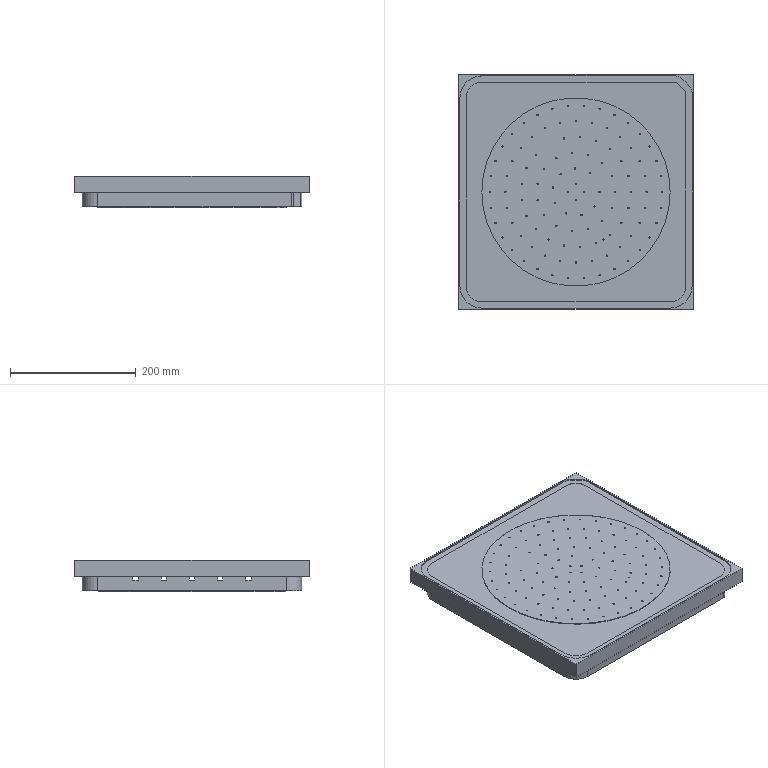Part | 4 solids | 704 faces | box 374 x 374 x 49.5 mm | volume 5747561 mm3 | cylinder 401 | plane 303 | commonest cylinder face diameters 2 x222 216.7 x20 233.3 x20 266.7 x20 283.3 x20 183.3 x16